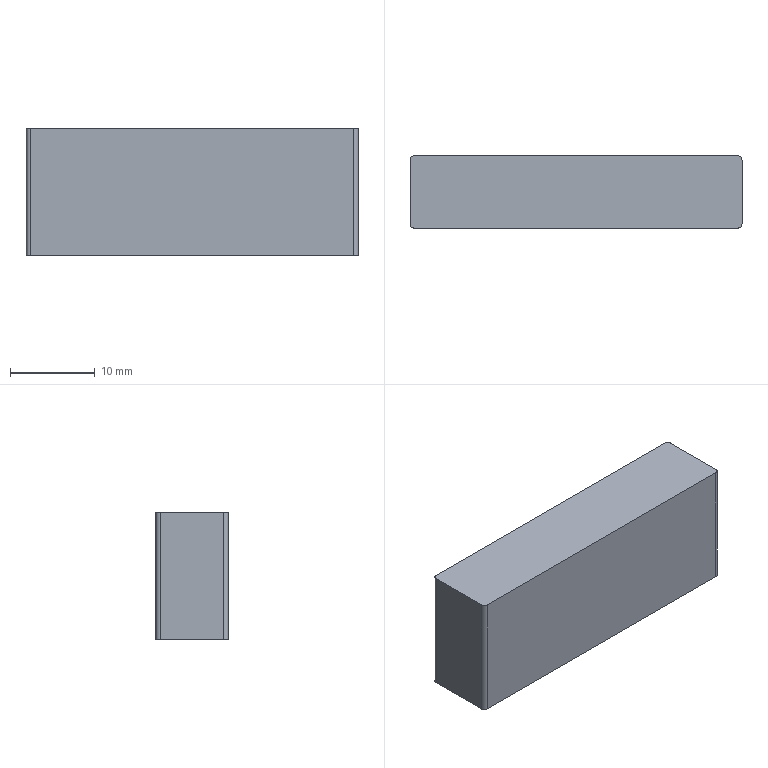Part | NX | features BREP 1 | 1 solid | 10 faces | box 39.1 x 8.507 x 15 mm | volume 4986 mm3 | plane 6 | cylinder 4 | commonest cylinder face diameters 1 x4
STEP:
#1=CARTESIAN_POINT('',(-19.05,4.254,-25.6));
#2=VERTEX_POINT('',#1);
#3=CARTESIAN_POINT('',(-19.55,3.754,-25.6));
#4=VERTEX_POINT('',#3);
#5=CARTESIAN_POINT('',(-19.05,3.754,-25.6));
#6=DIRECTION('',(0.,0.,1.));
#7=DIRECTION('',(1.,0.,0.));
#8=AXIS2_PLACEMENT_3D('',#5,#6,#7);
#9=CIRCLE('',#8,0.5);
#10=EDGE_CURVE('',#2,#4,#9,.T.);
#11=ORIENTED_EDGE('',*,*,#10,.F.);
#12=CARTESIAN_POINT('',(-19.05,4.254,-40.6));
#13=VERTEX_POINT('',#12);
#14=CARTESIAN_POINT('',(-19.05,4.254,-40.6));
#15=DIRECTION('',(0.,0.,1.));
#16=VECTOR('',#15,1000.);
#17=LINE('',#14,#16);
#18=EDGE_CURVE('',#13,#2,#17,.T.);
#19=ORIENTED_EDGE('',*,*,#18,.F.);
#20=CARTESIAN_POINT('',(-19.55,3.754,-40.6));
#21=VERTEX_POINT('',#20);
#22=CARTESIAN_POINT('',(-19.05,3.754,-40.6));
#23=DIRECTION('',(0.,0.,1.));
#24=DIRECTION('',(1.,0.,0.));
#25=AXIS2_PLACEMENT_3D('',#22,#23,#24);
#26=CIRCLE('',#25,0.5);
#27=EDGE_CURVE('',#13,#21,#26,.T.);
#28=ORIENTED_EDGE('',*,*,#27,.T.);
#29=CARTESIAN_POINT('',(-19.55,3.754,-40.6));
#30=DIRECTION('',(0.,0.,1.));
#31=VECTOR('',#30,1000.);
#32=LINE('',#29,#31);
#33=EDGE_CURVE('',#21,#4,#32,.T.);
#34=ORIENTED_EDGE('',*,*,#33,.T.);
#35=EDGE_LOOP('',(#11,#19,#28,#34));
#36=FACE_BOUND('',#35,.T.);
#37=CARTESIAN_POINT('',(-19.05,3.754,-40.6));
#38=DIRECTION('',(0.,0.,1.));
#39=DIRECTION('',(-1.,0.,0.));
#40=AXIS2_PLACEMENT_3D('',#37,#38,#39);
#41=CYLINDRICAL_SURFACE('',#40,0.5);
#42=ADVANCED_FACE('',(#36),#41,.T.);
#43=CARTESIAN_POINT('',(-19.55,-3.754,-25.6));
#44=VERTEX_POINT('',#43);
#45=CARTESIAN_POINT('',(-19.55,-3.754,-25.6));
#46=DIRECTION('',(0.,1.,0.));
#47=VECTOR('',#46,1000.);
#48=LINE('',#45,#47);
#49=EDGE_CURVE('',#44,#4,#48,.T.);
#50=ORIENTED_EDGE('',*,*,#49,.T.);
#51=ORIENTED_EDGE('',*,*,#33,.F.);
#52=CARTESIAN_POINT('',(-19.55,-3.754,-40.6));
#53=VERTEX_POINT('',#52);
#54=CARTESIAN_POINT('',(-19.55,-3.754,-40.6));
#55=DIRECTION('',(0.,1.,0.));
#56=VECTOR('',#55,1000.);
#57=LINE('',#54,#56);
#58=EDGE_CURVE('',#53,#21,#57,.T.);
#59=ORIENTED_EDGE('',*,*,#58,.F.);
#60=CARTESIAN_POINT('',(-19.55,-3.754,-40.6));
#61=DIRECTION('',(0.,0.,1.));
#62=VECTOR('',#61,1000.);
#63=LINE('',#60,#62);
#64=EDGE_CURVE('',#53,#44,#63,.T.);
#65=ORIENTED_EDGE('',*,*,#64,.T.);
#66=EDGE_LOOP('',(#50,#51,#59,#65));
#67=FACE_BOUND('',#66,.T.);
#68=CARTESIAN_POINT('',(-19.55,-3.754,-40.6));
#69=DIRECTION('',(1.,0.,0.));
#70=DIRECTION('',(0.,-1.,0.));
#71=AXIS2_PLACEMENT_3D('',#68,#69,#70);
#72=PLANE('',#71);
#73=ADVANCED_FACE('',(#67),#72,.F.);
#74=CARTESIAN_POINT('',(-19.05,-4.254,-25.6));
#75=VERTEX_POINT('',#74);
#76=CARTESIAN_POINT('',(-19.05,-3.754,-25.6));
#77=DIRECTION('',(0.,0.,1.));
#78=DIRECTION('',(1.,0.,0.));
#79=AXIS2_PLACEMENT_3D('',#76,#77,#78);
#80=CIRCLE('',#79,0.5);
#81=EDGE_CURVE('',#44,#75,#80,.T.);
#82=ORIENTED_EDGE('',*,*,#81,.F.);
#83=ORIENTED_EDGE('',*,*,#64,.F.);
#84=CARTESIAN_POINT('',(-19.05,-4.254,-40.6));
#85=VERTEX_POINT('',#84);
#86=CARTESIAN_POINT('',(-19.05,-3.754,-40.6));
#87=DIRECTION('',(0.,0.,1.));
#88=DIRECTION('',(1.,0.,0.));
#89=AXIS2_PLACEMENT_3D('',#86,#87,#88);
#90=CIRCLE('',#89,0.5);
#91=EDGE_CURVE('',#53,#85,#90,.T.);
#92=ORIENTED_EDGE('',*,*,#91,.T.);
#93=CARTESIAN_POINT('',(-19.05,-4.254,-40.6));
#94=DIRECTION('',(0.,0.,1.));
#95=VECTOR('',#94,1000.);
#96=LINE('',#93,#95);
#97=EDGE_CURVE('',#85,#75,#96,.T.);
#98=ORIENTED_EDGE('',*,*,#97,.T.);
#99=EDGE_LOOP('',(#82,#83,#92,#98));
#100=FACE_BOUND('',#99,.T.);
#101=CARTESIAN_POINT('',(-19.05,-3.754,-40.6));
#102=DIRECTION('',(0.,0.,1.));
#103=DIRECTION('',(-1.,0.,0.));
#104=AXIS2_PLACEMENT_3D('',#101,#102,#103);
#105=CYLINDRICAL_SURFACE('',#104,0.5);
#106=ADVANCED_FACE('',(#100),#105,.T.);
#107=CARTESIAN_POINT('',(19.05,-4.254,-25.6));
#108=VERTEX_POINT('',#107);
#109=CARTESIAN_POINT('',(19.05,-4.254,-25.6));
#110=DIRECTION('',(-1.,0.,0.));
#111=VECTOR('',#110,1000.);
#112=LINE('',#109,#111);
#113=EDGE_CURVE('',#108,#75,#112,.T.);
#114=ORIENTED_EDGE('',*,*,#113,.T.);
#115=ORIENTED_EDGE('',*,*,#97,.F.);
#116=CARTESIAN_POINT('',(19.05,-4.254,-40.6));
#117=VERTEX_POINT('',#116);
#118=CARTESIAN_POINT('',(19.05,-4.254,-40.6));
#119=DIRECTION('',(-1.,0.,0.));
#120=VECTOR('',#119,1000.);
#121=LINE('',#118,#120);
#122=EDGE_CURVE('',#117,#85,#121,.T.);
#123=ORIENTED_EDGE('',*,*,#122,.F.);
#124=CARTESIAN_POINT('',(19.05,-4.254,-40.6));
#125=DIRECTION('',(0.,0.,1.));
#126=VECTOR('',#125,1000.);
#127=LINE('',#124,#126);
#128=EDGE_CURVE('',#117,#108,#127,.T.);
#129=ORIENTED_EDGE('',*,*,#128,.T.);
#130=EDGE_LOOP('',(#114,#115,#123,#129));
#131=FACE_BOUND('',#130,.T.);
#132=CARTESIAN_POINT('',(19.05,-4.254,-40.6));
#133=DIRECTION('',(0.,1.,0.));
#134=DIRECTION('',(1.,0.,0.));
#135=AXIS2_PLACEMENT_3D('',#132,#133,#134);
#136=PLANE('',#135);
#137=ADVANCED_FACE('',(#131),#136,.F.);
#138=CARTESIAN_POINT('',(19.55,-3.754,-25.6));
#139=VERTEX_POINT('',#138);
#140=CARTESIAN_POINT('',(19.05,-3.754,-25.6));
#141=DIRECTION('',(0.,0.,1.));
#142=DIRECTION('',(1.,0.,0.));
#143=AXIS2_PLACEMENT_3D('',#140,#141,#142);
#144=CIRCLE('',#143,0.5);
#145=EDGE_CURVE('',#108,#139,#144,.T.);
#146=ORIENTED_EDGE('',*,*,#145,.F.);
#147=ORIENTED_EDGE('',*,*,#128,.F.);
#148=CARTESIAN_POINT('',(19.55,-3.754,-40.6));
#149=VERTEX_POINT('',#148);
#150=CARTESIAN_POINT('',(19.05,-3.754,-40.6));
#151=DIRECTION('',(0.,0.,1.));
#152=DIRECTION('',(1.,0.,0.));
#153=AXIS2_PLACEMENT_3D('',#150,#151,#152);
#154=CIRCLE('',#153,0.5);
#155=EDGE_CURVE('',#117,#149,#154,.T.);
#156=ORIENTED_EDGE('',*,*,#155,.T.);
#157=CARTESIAN_POINT('',(19.55,-3.754,-40.6));
#158=DIRECTION('',(0.,0.,1.));
#159=VECTOR('',#158,1000.);
#160=LINE('',#157,#159);
#161=EDGE_CURVE('',#149,#139,#160,.T.);
#162=ORIENTED_EDGE('',*,*,#161,.T.);
#163=EDGE_LOOP('',(#146,#147,#156,#162));
#164=FACE_BOUND('',#163,.T.);
#165=CARTESIAN_POINT('',(19.05,-3.754,-40.6));
#166=DIRECTION('',(0.,0.,1.));
#167=DIRECTION('',(-1.,0.,0.));
#168=AXIS2_PLACEMENT_3D('',#165,#166,#167);
#169=CYLINDRICAL_SURFACE('',#168,0.5);
#170=ADVANCED_FACE('',(#164),#169,.T.);
#171=CARTESIAN_POINT('',(19.55,3.754,-25.6));
#172=VERTEX_POINT('',#171);
#173=CARTESIAN_POINT('',(19.55,3.754,-25.6));
#174=DIRECTION('',(0.,-1.,0.));
#175=VECTOR('',#174,1000.);
#176=LINE('',#173,#175);
#177=EDGE_CURVE('',#172,#139,#176,.T.);
#178=ORIENTED_EDGE('',*,*,#177,.T.);
#179=ORIENTED_EDGE('',*,*,#161,.F.);
#180=CARTESIAN_POINT('',(19.55,3.754,-40.6));
#181=VERTEX_POINT('',#180);
#182=CARTESIAN_POINT('',(19.55,3.754,-40.6));
#183=DIRECTION('',(0.,-1.,0.));
#184=VECTOR('',#183,1000.);
#185=LINE('',#182,#184);
#186=EDGE_CURVE('',#181,#149,#185,.T.);
#187=ORIENTED_EDGE('',*,*,#186,.F.);
#188=CARTESIAN_POINT('',(19.55,3.754,-40.6));
#189=DIRECTION('',(0.,0.,1.));
#190=VECTOR('',#189,1000.);
#191=LINE('',#188,#190);
#192=EDGE_CURVE('',#181,#172,#191,.T.);
#193=ORIENTED_EDGE('',*,*,#192,.T.);
#194=EDGE_LOOP('',(#178,#179,#187,#193));
#195=FACE_BOUND('',#194,.T.);
#196=CARTESIAN_POINT('',(19.55,3.754,-40.6));
#197=DIRECTION('',(-1.,0.,0.));
#198=DIRECTION('',(0.,1.,0.));
#199=AXIS2_PLACEMENT_3D('',#196,#197,#198);
#200=PLANE('',#199);
#201=ADVANCED_FACE('',(#195),#200,.F.);
#202=CARTESIAN_POINT('',(19.05,4.254,-25.6));
#203=VERTEX_POINT('',#202);
#204=CARTESIAN_POINT('',(19.05,3.754,-25.6));
#205=DIRECTION('',(0.,0.,1.));
#206=DIRECTION('',(1.,0.,0.));
#207=AXIS2_PLACEMENT_3D('',#204,#205,#206);
#208=CIRCLE('',#207,0.5);
#209=EDGE_CURVE('',#172,#203,#208,.T.);
#210=ORIENTED_EDGE('',*,*,#209,.F.);
#211=ORIENTED_EDGE('',*,*,#192,.F.);
#212=CARTESIAN_POINT('',(19.05,4.254,-40.6));
#213=VERTEX_POINT('',#212);
#214=CARTESIAN_POINT('',(19.05,3.754,-40.6));
#215=DIRECTION('',(0.,0.,1.));
#216=DIRECTION('',(1.,0.,0.));
#217=AXIS2_PLACEMENT_3D('',#214,#215,#216);
#218=CIRCLE('',#217,0.5);
#219=EDGE_CURVE('',#181,#213,#218,.T.);
#220=ORIENTED_EDGE('',*,*,#219,.T.);
#221=CARTESIAN_POINT('',(19.05,4.254,-40.6));
#222=DIRECTION('',(0.,0.,1.));
#223=VECTOR('',#222,1000.);
#224=LINE('',#221,#223);
#225=EDGE_CURVE('',#213,#203,#224,.T.);
#226=ORIENTED_EDGE('',*,*,#225,.T.);
#227=EDGE_LOOP('',(#210,#211,#220,#226));
#228=FACE_BOUND('',#227,.T.);
#229=CARTESIAN_POINT('',(19.05,3.754,-40.6));
#230=DIRECTION('',(0.,0.,1.));
#231=DIRECTION('',(-1.,0.,0.));
#232=AXIS2_PLACEMENT_3D('',#229,#230,#231);
#233=CYLINDRICAL_SURFACE('',#232,0.5);
#234=ADVANCED_FACE('',(#228),#233,.T.);
#235=CARTESIAN_POINT('',(-19.05,4.254,-25.6));
#236=DIRECTION('',(1.,0.,0.));
#237=VECTOR('',#236,1000.);
#238=LINE('',#235,#237);
#239=EDGE_CURVE('',#2,#203,#238,.T.);
#240=ORIENTED_EDGE('',*,*,#239,.T.);
#241=ORIENTED_EDGE('',*,*,#225,.F.);
#242=CARTESIAN_POINT('',(-19.05,4.254,-40.6));
#243=DIRECTION('',(1.,0.,0.));
#244=VECTOR('',#243,1000.);
#245=LINE('',#242,#244);
#246=EDGE_CURVE('',#13,#213,#245,.T.);
#247=ORIENTED_EDGE('',*,*,#246,.F.);
#248=ORIENTED_EDGE('',*,*,#18,.T.);
#249=EDGE_LOOP('',(#240,#241,#247,#248));
#250=FACE_BOUND('',#249,.T.);
#251=CARTESIAN_POINT('',(-19.05,4.254,-40.6));
#252=DIRECTION('',(0.,-1.,0.));
#253=DIRECTION('',(0.,0.,1.));
#254=AXIS2_PLACEMENT_3D('',#251,#252,#253);
#255=PLANE('',#254);
#256=ADVANCED_FACE('',(#250),#255,.F.);
#257=ORIENTED_EDGE('',*,*,#27,.F.);
#258=ORIENTED_EDGE('',*,*,#246,.T.);
#259=ORIENTED_EDGE('',*,*,#219,.F.);
#260=ORIENTED_EDGE('',*,*,#186,.T.);
#261=ORIENTED_EDGE('',*,*,#155,.F.);
#262=ORIENTED_EDGE('',*,*,#122,.T.);
#263=ORIENTED_EDGE('',*,*,#91,.F.);
#264=ORIENTED_EDGE('',*,*,#58,.T.);
#265=EDGE_LOOP('',(#257,#258,#259,#260,#261,#262,#263,#264));
#266=FACE_BOUND('',#265,.T.);
#267=CARTESIAN_POINT('',(-19.05,3.754,-40.6));
#268=DIRECTION('',(0.,0.,1.));
#269=DIRECTION('',(-1.,0.,0.));
#270=AXIS2_PLACEMENT_3D('',#267,#268,#269);
#271=PLANE('',#270);
#272=ADVANCED_FACE('',(#266),#271,.F.);
#273=ORIENTED_EDGE('',*,*,#10,.T.);
#274=ORIENTED_EDGE('',*,*,#49,.F.);
#275=ORIENTED_EDGE('',*,*,#81,.T.);
#276=ORIENTED_EDGE('',*,*,#113,.F.);
#277=ORIENTED_EDGE('',*,*,#145,.T.);
#278=ORIENTED_EDGE('',*,*,#177,.F.);
#279=ORIENTED_EDGE('',*,*,#209,.T.);
#280=ORIENTED_EDGE('',*,*,#239,.F.);
#281=EDGE_LOOP('',(#273,#274,#275,#276,#277,#278,#279,#280));
#282=FACE_BOUND('',#281,.T.);
#283=CARTESIAN_POINT('',(-19.05,3.754,-25.6));
#284=DIRECTION('',(0.,0.,1.));
#285=DIRECTION('',(-1.,0.,0.));
#286=AXIS2_PLACEMENT_3D('',#283,#284,#285);
#287=PLANE('',#286);
#288=ADVANCED_FACE('',(#282),#287,.T.);
#289=CLOSED_SHELL('',(#42,#73,#106,#137,#170,#201,#234,#256,#272,#288));
#290=MANIFOLD_SOLID_BREP('',#289);
#291=(LENGTH_UNIT()NAMED_UNIT(*)SI_UNIT(.MILLI.,.METRE.));
#292=UNCERTAINTY_MEASURE_WITH_UNIT(LENGTH_MEASURE(0.00001),#291,'','');
#293=(NAMED_UNIT(*)PLANE_ANGLE_UNIT()SI_UNIT($,.RADIAN.));
#294=(NAMED_UNIT(*)SI_UNIT($,.STERADIAN.)SOLID_ANGLE_UNIT());
#295=(GEOMETRIC_REPRESENTATION_CONTEXT(3)GLOBAL_UNCERTAINTY_ASSIGNED_CONTEXT((#292))GLOBAL_UNIT_ASSIGNED_CONTEXT((#291,#293,#294))REPRESENTATION_CONTEXT('',''));
#296=ADVANCED_BREP_SHAPE_REPRESENTATION('',(#290),#295);